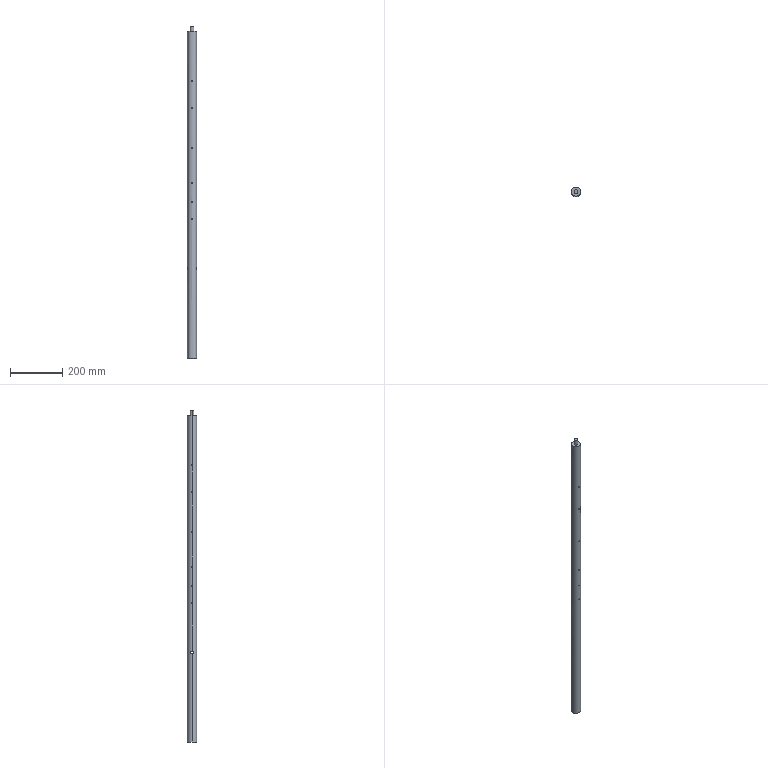Part | SolidWorks | features ICE 5, LPattern 4, 3DProfileFeature 2, CirPattern 2, HoleWzd 2, Chamfer 1, Extrusion 1 | 1 solid | 105 faces | box 35 x 35 x 1273 mm | volume 1203146 mm3 | cylinder 54 | cone 48 | plane 3 | commonest cylinder face diameters 3.3 x24 4.2 x24 10 x2 15 x2 35 x2